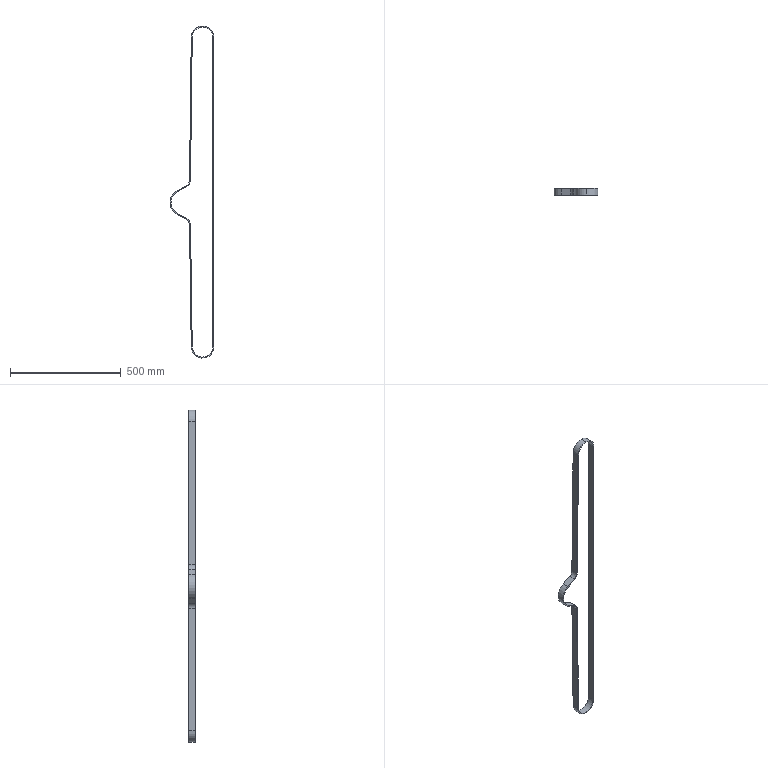Part | SolidWorks | features ExtruThin 1 | 1 solid | 24 faces | box 198.54 x 30 x 1498 mm | volume 429965 mm3 | cylinder 12 | plane 12 | commonest cylinder face diameters 93.49 x3 102.49 x3 55 x2 64 x2 112.59 x1 121.59 x1
STEP:
#1=CARTESIAN_POINT('',(-7.645,219.46,1948.));
#2=VERTEX_POINT('',#1);
#3=CARTESIAN_POINT('',(-54.39,219.46,1994.745));
#4=VERTEX_POINT('',#3);
#5=CARTESIAN_POINT('',(-54.39,219.46,1948.));
#6=DIRECTION('',(0.,-1.,0.));
#7=DIRECTION('',(0.,0.,1.));
#8=AXIS2_PLACEMENT_3D('',#5,#6,#7);
#9=CIRCLE('',#8,46.745);
#10=EDGE_CURVE('',#2,#4,#9,.T.);
#11=ORIENTED_EDGE('',*,*,#10,.T.);
#12=CARTESIAN_POINT('',(-54.39,249.46,1994.745));
#13=VERTEX_POINT('',#12);
#14=CARTESIAN_POINT('',(-54.39,219.46,1994.745));
#15=DIRECTION('',(0.,1.,0.));
#16=VECTOR('',#15,1000.);
#17=LINE('',#14,#16);
#18=EDGE_CURVE('',#4,#13,#17,.T.);
#19=ORIENTED_EDGE('',*,*,#18,.T.);
#20=CARTESIAN_POINT('',(-7.645,249.46,1948.));
#21=VERTEX_POINT('',#20);
#22=CARTESIAN_POINT('',(-54.39,249.46,1948.));
#23=DIRECTION('',(0.,-1.,0.));
#24=DIRECTION('',(0.,0.,1.));
#25=AXIS2_PLACEMENT_3D('',#22,#23,#24);
#26=CIRCLE('',#25,46.745);
#27=EDGE_CURVE('',#21,#13,#26,.T.);
#28=ORIENTED_EDGE('',*,*,#27,.F.);
#29=CARTESIAN_POINT('',(-7.645,219.46,1948.));
#30=DIRECTION('',(0.,1.,0.));
#31=VECTOR('',#30,1000.);
#32=LINE('',#29,#31);
#33=EDGE_CURVE('',#2,#21,#32,.T.);
#34=ORIENTED_EDGE('',*,*,#33,.F.);
#35=EDGE_LOOP('',(#11,#19,#28,#34));
#36=FACE_OUTER_BOUND('',#35,.T.);
#37=CARTESIAN_POINT('',(-54.39,219.46,1948.));
#38=DIRECTION('',(0.,1.,0.));
#39=DIRECTION('',(0.,0.,1.));
#40=AXIS2_PLACEMENT_3D('',#37,#38,#39);
#41=CYLINDRICAL_SURFACE('',#40,46.745);
#42=ADVANCED_FACE('',(#36),#41,.F.);
#43=CARTESIAN_POINT('',(-54.39,219.46,1999.245));
#44=VERTEX_POINT('',#43);
#45=CARTESIAN_POINT('',(-105.631,219.46,1948.615));
#46=VERTEX_POINT('',#45);
#47=CARTESIAN_POINT('',(-54.39,219.46,1948.));
#48=DIRECTION('',(0.,-1.,0.));
#49=DIRECTION('',(0.,0.,1.));
#50=AXIS2_PLACEMENT_3D('',#47,#48,#49);
#51=CIRCLE('',#50,51.245);
#52=EDGE_CURVE('',#44,#46,#51,.T.);
#53=ORIENTED_EDGE('',*,*,#52,.F.);
#54=CARTESIAN_POINT('',(-54.39,249.46,1999.245));
#55=VERTEX_POINT('',#54);
#56=CARTESIAN_POINT('',(-54.39,219.46,1999.245));
#57=DIRECTION('',(0.,1.,0.));
#58=VECTOR('',#57,1000.);
#59=LINE('',#56,#58);
#60=EDGE_CURVE('',#44,#55,#59,.T.);
#61=ORIENTED_EDGE('',*,*,#60,.T.);
#62=CARTESIAN_POINT('',(-105.631,249.46,1948.615));
#63=VERTEX_POINT('',#62);
#64=CARTESIAN_POINT('',(-54.39,249.46,1948.));
#65=DIRECTION('',(0.,-1.,0.));
#66=DIRECTION('',(0.,0.,1.));
#67=AXIS2_PLACEMENT_3D('',#64,#65,#66);
#68=CIRCLE('',#67,51.245);
#69=EDGE_CURVE('',#55,#63,#68,.T.);
#70=ORIENTED_EDGE('',*,*,#69,.T.);
#71=CARTESIAN_POINT('',(-105.631,219.46,1948.615));
#72=DIRECTION('',(0.,1.,0.));
#73=VECTOR('',#72,1000.);
#74=LINE('',#71,#73);
#75=EDGE_CURVE('',#46,#63,#74,.T.);
#76=ORIENTED_EDGE('',*,*,#75,.F.);
#77=EDGE_LOOP('',(#53,#61,#70,#76));
#78=FACE_OUTER_BOUND('',#77,.T.);
#79=CARTESIAN_POINT('',(-54.39,219.46,1948.));
#80=DIRECTION('',(0.,1.,0.));
#81=DIRECTION('',(0.,0.,1.));
#82=AXIS2_PLACEMENT_3D('',#79,#80,#81);
#83=CYLINDRICAL_SURFACE('',#82,51.245);
#84=ADVANCED_FACE('',(#78),#83,.T.);
#85=CARTESIAN_POINT('',(-105.63,219.46,551.279));
#86=VERTEX_POINT('',#85);
#87=CARTESIAN_POINT('',(-3.145,219.46,552.));
#88=VERTEX_POINT('',#87);
#89=CARTESIAN_POINT('',(-54.39,219.46,552.));
#90=DIRECTION('',(0.,-1.,0.));
#91=DIRECTION('',(0.,0.,1.));
#92=AXIS2_PLACEMENT_3D('',#89,#90,#91);
#93=CIRCLE('',#92,51.245);
#94=EDGE_CURVE('',#86,#88,#93,.T.);
#95=ORIENTED_EDGE('',*,*,#94,.T.);
#96=CARTESIAN_POINT('',(-3.145,219.46,1948.));
#97=VERTEX_POINT('',#96);
#98=CARTESIAN_POINT('',(-3.145,219.46,552.));
#99=DIRECTION('',(0.,0.,1.));
#100=VECTOR('',#99,1000.);
#101=LINE('',#98,#100);
#102=EDGE_CURVE('',#88,#97,#101,.T.);
#103=ORIENTED_EDGE('',*,*,#102,.T.);
#104=CARTESIAN_POINT('',(-54.39,219.46,1948.));
#105=DIRECTION('',(0.,-1.,0.));
#106=DIRECTION('',(0.,0.,1.));
#107=AXIS2_PLACEMENT_3D('',#104,#105,#106);
#108=CIRCLE('',#107,51.245);
#109=EDGE_CURVE('',#97,#44,#108,.T.);
#110=ORIENTED_EDGE('',*,*,#109,.T.);
#111=ORIENTED_EDGE('',*,*,#52,.T.);
#112=CARTESIAN_POINT('',(-113.392,219.46,1302.17));
#113=VERTEX_POINT('',#112);
#114=CARTESIAN_POINT('',(-105.631,219.46,1948.615));
#115=DIRECTION('',(-0.012,0.,-0.9999));
#116=VECTOR('',#115,1000.);
#117=LINE('',#114,#116);
#118=EDGE_CURVE('',#46,#113,#117,.T.);
#119=ORIENTED_EDGE('',*,*,#118,.T.);
#120=CARTESIAN_POINT('',(-127.979,219.46,1278.219));
#121=VERTEX_POINT('',#120);
#122=CARTESIAN_POINT('',(-140.89,219.46,1302.5));
#123=DIRECTION('',(0.,1.,0.));
#124=DIRECTION('',(0.,0.,1.));
#125=AXIS2_PLACEMENT_3D('',#122,#123,#124);
#126=CIRCLE('',#125,27.5);
#127=EDGE_CURVE('',#113,#121,#126,.T.);
#128=ORIENTED_EDGE('',*,*,#127,.T.);
#129=CARTESIAN_POINT('',(-169.431,219.46,1256.179));
#130=VERTEX_POINT('',#129);
#131=CARTESIAN_POINT('',(-169.431,219.46,1256.179));
#132=DIRECTION('',(-0.8829,0.,-0.4695));
#133=VECTOR('',#132,1000.);
#134=LINE('',#131,#133);
#135=EDGE_CURVE('',#121,#130,#134,.T.);
#136=ORIENTED_EDGE('',*,*,#135,.T.);
#137=CARTESIAN_POINT('',(-169.431,219.46,1148.821));
#138=VERTEX_POINT('',#137);
#139=CARTESIAN_POINT('',(-140.89,219.46,1202.5));
#140=DIRECTION('',(0.,-1.,0.));
#141=DIRECTION('',(0.,0.,1.));
#142=AXIS2_PLACEMENT_3D('',#139,#140,#141);
#143=CIRCLE('',#142,60.795);
#144=EDGE_CURVE('',#130,#138,#143,.T.);
#145=ORIENTED_EDGE('',*,*,#144,.T.);
#146=CARTESIAN_POINT('',(-127.979,219.46,1126.781));
#147=VERTEX_POINT('',#146);
#148=CARTESIAN_POINT('',(-127.979,219.46,1126.781));
#149=DIRECTION('',(0.883,0.,-0.4695));
#150=VECTOR('',#149,1000.);
#151=LINE('',#148,#150);
#152=EDGE_CURVE('',#138,#147,#151,.T.);
#153=ORIENTED_EDGE('',*,*,#152,.T.);
#154=CARTESIAN_POINT('',(-113.393,219.46,1102.887));
#155=VERTEX_POINT('',#154);
#156=CARTESIAN_POINT('',(-140.89,219.46,1102.5));
#157=DIRECTION('',(0.,1.,0.));
#158=DIRECTION('',(0.,0.,1.));
#159=AXIS2_PLACEMENT_3D('',#156,#157,#158);
#160=CIRCLE('',#159,27.5);
#161=EDGE_CURVE('',#147,#155,#160,.T.);
#162=ORIENTED_EDGE('',*,*,#161,.T.);
#163=CARTESIAN_POINT('',(-105.63,219.46,551.279));
#164=DIRECTION('',(0.01407,0.,-0.9999));
#165=VECTOR('',#164,1000.);
#166=LINE('',#163,#165);
#167=EDGE_CURVE('',#155,#86,#166,.T.);
#168=ORIENTED_EDGE('',*,*,#167,.T.);
#169=EDGE_LOOP('',(#95,#103,#110,#111,#119,#128,#136,#145,#153,#162,#168));
#170=FACE_OUTER_BOUND('',#169,.T.);
#171=CARTESIAN_POINT('',(-7.645,219.46,552.));
#172=VERTEX_POINT('',#171);
#173=CARTESIAN_POINT('',(-7.645,219.46,552.));
#174=DIRECTION('',(0.,0.,1.));
#175=VECTOR('',#174,1000.);
#176=LINE('',#173,#175);
#177=EDGE_CURVE('',#172,#2,#176,.T.);
#178=ORIENTED_EDGE('',*,*,#177,.F.);
#179=CARTESIAN_POINT('',(-101.13,219.46,551.342));
#180=VERTEX_POINT('',#179);
#181=CARTESIAN_POINT('',(-54.39,219.46,552.));
#182=DIRECTION('',(0.,-1.,0.));
#183=DIRECTION('',(0.,0.,1.));
#184=AXIS2_PLACEMENT_3D('',#181,#182,#183);
#185=CIRCLE('',#184,46.745);
#186=EDGE_CURVE('',#180,#172,#185,.T.);
#187=ORIENTED_EDGE('',*,*,#186,.F.);
#188=CARTESIAN_POINT('',(-108.893,219.46,1102.95));
#189=VERTEX_POINT('',#188);
#190=CARTESIAN_POINT('',(-101.13,219.46,551.342));
#191=DIRECTION('',(0.01407,0.,-0.9999));
#192=VECTOR('',#191,1000.);
#193=LINE('',#190,#192);
#194=EDGE_CURVE('',#189,#180,#193,.T.);
#195=ORIENTED_EDGE('',*,*,#194,.F.);
#196=CARTESIAN_POINT('',(-125.867,219.46,1130.754));
#197=VERTEX_POINT('',#196);
#198=CARTESIAN_POINT('',(-140.89,219.46,1102.5));
#199=DIRECTION('',(0.,1.,0.));
#200=DIRECTION('',(0.,0.,1.));
#201=AXIS2_PLACEMENT_3D('',#198,#199,#200);
#202=CIRCLE('',#201,32.);
#203=EDGE_CURVE('',#197,#189,#202,.T.);
#204=ORIENTED_EDGE('',*,*,#203,.F.);
#205=CARTESIAN_POINT('',(-167.318,219.46,1152.794));
#206=VERTEX_POINT('',#205);
#207=CARTESIAN_POINT('',(-125.867,219.46,1130.754));
#208=DIRECTION('',(0.883,0.,-0.4695));
#209=VECTOR('',#208,1000.);
#210=LINE('',#207,#209);
#211=EDGE_CURVE('',#206,#197,#210,.T.);
#212=ORIENTED_EDGE('',*,*,#211,.F.);
#213=CARTESIAN_POINT('',(-167.318,219.46,1252.206));
#214=VERTEX_POINT('',#213);
#215=CARTESIAN_POINT('',(-140.89,219.46,1202.5));
#216=DIRECTION('',(0.,-1.,0.));
#217=DIRECTION('',(0.,0.,1.));
#218=AXIS2_PLACEMENT_3D('',#215,#216,#217);
#219=CIRCLE('',#218,56.295);
#220=EDGE_CURVE('',#214,#206,#219,.T.);
#221=ORIENTED_EDGE('',*,*,#220,.F.);
#222=CARTESIAN_POINT('',(-125.867,219.46,1274.246));
#223=VERTEX_POINT('',#222);
#224=CARTESIAN_POINT('',(-167.318,219.46,1252.206));
#225=DIRECTION('',(-0.8829,0.,-0.4695));
#226=VECTOR('',#225,1000.);
#227=LINE('',#224,#226);
#228=EDGE_CURVE('',#223,#214,#227,.T.);
#229=ORIENTED_EDGE('',*,*,#228,.F.);
#230=CARTESIAN_POINT('',(-108.892,219.46,1302.116));
#231=VERTEX_POINT('',#230);
#232=CARTESIAN_POINT('',(-140.89,219.46,1302.5));
#233=DIRECTION('',(0.,1.,0.));
#234=DIRECTION('',(0.,0.,1.));
#235=AXIS2_PLACEMENT_3D('',#232,#233,#234);
#236=CIRCLE('',#235,32.);
#237=EDGE_CURVE('',#231,#223,#236,.T.);
#238=ORIENTED_EDGE('',*,*,#237,.F.);
#239=CARTESIAN_POINT('',(-101.131,219.46,1948.561));
#240=VERTEX_POINT('',#239);
#241=CARTESIAN_POINT('',(-101.131,219.46,1948.561));
#242=DIRECTION('',(-0.012,0.,-0.9999));
#243=VECTOR('',#242,1000.);
#244=LINE('',#241,#243);
#245=EDGE_CURVE('',#240,#231,#244,.T.);
#246=ORIENTED_EDGE('',*,*,#245,.F.);
#247=CARTESIAN_POINT('',(-54.39,219.46,1948.));
#248=DIRECTION('',(0.,-1.,0.));
#249=DIRECTION('',(0.,0.,1.));
#250=AXIS2_PLACEMENT_3D('',#247,#248,#249);
#251=CIRCLE('',#250,46.745);
#252=EDGE_CURVE('',#4,#240,#251,.T.);
#253=ORIENTED_EDGE('',*,*,#252,.F.);
#254=ORIENTED_EDGE('',*,*,#10,.F.);
#255=EDGE_LOOP('',(#178,#187,#195,#204,#212,#221,#229,#238,#246,#253,#254));
#256=FACE_BOUND('',#255,.T.);
#257=CARTESIAN_POINT('',(-54.39,219.46,552.));
#258=DIRECTION('',(0.,-1.,0.));
#259=DIRECTION('',(0.,0.,-1.));
#260=AXIS2_PLACEMENT_3D('',#257,#258,#259);
#261=PLANE('',#260);
#262=ADVANCED_FACE('',(#170,#256),#261,.T.);
#263=CARTESIAN_POINT('',(-105.63,249.46,551.279));
#264=VERTEX_POINT('',#263);
#265=CARTESIAN_POINT('',(-3.145,249.46,552.));
#266=VERTEX_POINT('',#265);
#267=CARTESIAN_POINT('',(-54.39,249.46,552.));
#268=DIRECTION('',(0.,-1.,0.));
#269=DIRECTION('',(0.,0.,1.));
#270=AXIS2_PLACEMENT_3D('',#267,#268,#269);
#271=CIRCLE('',#270,51.245);
#272=EDGE_CURVE('',#264,#266,#271,.T.);
#273=ORIENTED_EDGE('',*,*,#272,.F.);
#274=CARTESIAN_POINT('',(-113.393,249.46,1102.887));
#275=VERTEX_POINT('',#274);
#276=CARTESIAN_POINT('',(-105.63,249.46,551.279));
#277=DIRECTION('',(0.01407,0.,-0.9999));
#278=VECTOR('',#277,1000.);
#279=LINE('',#276,#278);
#280=EDGE_CURVE('',#275,#264,#279,.T.);
#281=ORIENTED_EDGE('',*,*,#280,.F.);
#282=CARTESIAN_POINT('',(-127.979,249.46,1126.781));
#283=VERTEX_POINT('',#282);
#284=CARTESIAN_POINT('',(-140.89,249.46,1102.5));
#285=DIRECTION('',(0.,1.,0.));
#286=DIRECTION('',(0.,0.,1.));
#287=AXIS2_PLACEMENT_3D('',#284,#285,#286);
#288=CIRCLE('',#287,27.5);
#289=EDGE_CURVE('',#283,#275,#288,.T.);
#290=ORIENTED_EDGE('',*,*,#289,.F.);
#291=CARTESIAN_POINT('',(-169.431,249.46,1148.821));
#292=VERTEX_POINT('',#291);
#293=CARTESIAN_POINT('',(-127.979,249.46,1126.781));
#294=DIRECTION('',(0.883,0.,-0.4695));
#295=VECTOR('',#294,1000.);
#296=LINE('',#293,#295);
#297=EDGE_CURVE('',#292,#283,#296,.T.);
#298=ORIENTED_EDGE('',*,*,#297,.F.);
#299=CARTESIAN_POINT('',(-169.431,249.46,1256.179));
#300=VERTEX_POINT('',#299);
#301=CARTESIAN_POINT('',(-140.89,249.46,1202.5));
#302=DIRECTION('',(0.,-1.,0.));
#303=DIRECTION('',(0.,0.,1.));
#304=AXIS2_PLACEMENT_3D('',#301,#302,#303);
#305=CIRCLE('',#304,60.795);
#306=EDGE_CURVE('',#300,#292,#305,.T.);
#307=ORIENTED_EDGE('',*,*,#306,.F.);
#308=CARTESIAN_POINT('',(-127.979,249.46,1278.219));
#309=VERTEX_POINT('',#308);
#310=CARTESIAN_POINT('',(-169.431,249.46,1256.179));
#311=DIRECTION('',(-0.8829,0.,-0.4695));
#312=VECTOR('',#311,1000.);
#313=LINE('',#310,#312);
#314=EDGE_CURVE('',#309,#300,#313,.T.);
#315=ORIENTED_EDGE('',*,*,#314,.F.);
#316=CARTESIAN_POINT('',(-113.392,249.46,1302.17));
#317=VERTEX_POINT('',#316);
#318=CARTESIAN_POINT('',(-140.89,249.46,1302.5));
#319=DIRECTION('',(0.,1.,0.));
#320=DIRECTION('',(0.,0.,1.));
#321=AXIS2_PLACEMENT_3D('',#318,#319,#320);
#322=CIRCLE('',#321,27.5);
#323=EDGE_CURVE('',#317,#309,#322,.T.);
#324=ORIENTED_EDGE('',*,*,#323,.F.);
#325=CARTESIAN_POINT('',(-105.631,249.46,1948.615));
#326=DIRECTION('',(-0.012,0.,-0.9999));
#327=VECTOR('',#326,1000.);
#328=LINE('',#325,#327);
#329=EDGE_CURVE('',#63,#317,#328,.T.);
#330=ORIENTED_EDGE('',*,*,#329,.F.);
#331=ORIENTED_EDGE('',*,*,#69,.F.);
#332=CARTESIAN_POINT('',(-3.145,249.46,1948.));
#333=VERTEX_POINT('',#332);
#334=CARTESIAN_POINT('',(-54.39,249.46,1948.));
#335=DIRECTION('',(0.,-1.,0.));
#336=DIRECTION('',(0.,0.,1.));
#337=AXIS2_PLACEMENT_3D('',#334,#335,#336);
#338=CIRCLE('',#337,51.245);
#339=EDGE_CURVE('',#333,#55,#338,.T.);
#340=ORIENTED_EDGE('',*,*,#339,.F.);
#341=CARTESIAN_POINT('',(-3.145,249.46,552.));
#342=DIRECTION('',(0.,0.,1.));
#343=VECTOR('',#342,1000.);
#344=LINE('',#341,#343);
#345=EDGE_CURVE('',#266,#333,#344,.T.);
#346=ORIENTED_EDGE('',*,*,#345,.F.);
#347=EDGE_LOOP('',(#273,#281,#290,#298,#307,#315,#324,#330,#331,#340,#346));
#348=FACE_OUTER_BOUND('',#347,.T.);
#349=CARTESIAN_POINT('',(-101.13,249.46,551.342));
#350=VERTEX_POINT('',#349);
#351=CARTESIAN_POINT('',(-7.645,249.46,552.));
#352=VERTEX_POINT('',#351);
#353=CARTESIAN_POINT('',(-54.39,249.46,552.));
#354=DIRECTION('',(0.,-1.,0.));
#355=DIRECTION('',(0.,0.,1.));
#356=AXIS2_PLACEMENT_3D('',#353,#354,#355);
#357=CIRCLE('',#356,46.745);
#358=EDGE_CURVE('',#350,#352,#357,.T.);
#359=ORIENTED_EDGE('',*,*,#358,.T.);
#360=CARTESIAN_POINT('',(-7.645,249.46,552.));
#361=DIRECTION('',(0.,0.,1.));
#362=VECTOR('',#361,1000.);
#363=LINE('',#360,#362);
#364=EDGE_CURVE('',#352,#21,#363,.T.);
#365=ORIENTED_EDGE('',*,*,#364,.T.);
#366=ORIENTED_EDGE('',*,*,#27,.T.);
#367=CARTESIAN_POINT('',(-101.131,249.46,1948.561));
#368=VERTEX_POINT('',#367);
#369=CARTESIAN_POINT('',(-54.39,249.46,1948.));
#370=DIRECTION('',(0.,-1.,0.));
#371=DIRECTION('',(0.,0.,1.));
#372=AXIS2_PLACEMENT_3D('',#369,#370,#371);
#373=CIRCLE('',#372,46.745);
#374=EDGE_CURVE('',#13,#368,#373,.T.);
#375=ORIENTED_EDGE('',*,*,#374,.T.);
#376=CARTESIAN_POINT('',(-108.892,249.46,1302.116));
#377=VERTEX_POINT('',#376);
#378=CARTESIAN_POINT('',(-101.131,249.46,1948.561));
#379=DIRECTION('',(-0.012,0.,-0.9999));
#380=VECTOR('',#379,1000.);
#381=LINE('',#378,#380);
#382=EDGE_CURVE('',#368,#377,#381,.T.);
#383=ORIENTED_EDGE('',*,*,#382,.T.);
#384=CARTESIAN_POINT('',(-125.867,249.46,1274.246));
#385=VERTEX_POINT('',#384);
#386=CARTESIAN_POINT('',(-140.89,249.46,1302.5));
#387=DIRECTION('',(0.,1.,0.));
#388=DIRECTION('',(0.,0.,1.));
#389=AXIS2_PLACEMENT_3D('',#386,#387,#388);
#390=CIRCLE('',#389,32.);
#391=EDGE_CURVE('',#377,#385,#390,.T.);
#392=ORIENTED_EDGE('',*,*,#391,.T.);
#393=CARTESIAN_POINT('',(-167.318,249.46,1252.206));
#394=VERTEX_POINT('',#393);
#395=CARTESIAN_POINT('',(-167.318,249.46,1252.206));
#396=DIRECTION('',(-0.8829,0.,-0.4695));
#397=VECTOR('',#396,1000.);
#398=LINE('',#395,#397);
#399=EDGE_CURVE('',#385,#394,#398,.T.);
#400=ORIENTED_EDGE('',*,*,#399,.T.);
#401=CARTESIAN_POINT('',(-167.318,249.46,1152.794));
#402=VERTEX_POINT('',#401);
#403=CARTESIAN_POINT('',(-140.89,249.46,1202.5));
#404=DIRECTION('',(0.,-1.,0.));
#405=DIRECTION('',(0.,0.,1.));
#406=AXIS2_PLACEMENT_3D('',#403,#404,#405);
#407=CIRCLE('',#406,56.295);
#408=EDGE_CURVE('',#394,#402,#407,.T.);
#409=ORIENTED_EDGE('',*,*,#408,.T.);
#410=CARTESIAN_POINT('',(-125.867,249.46,1130.754));
#411=VERTEX_POINT('',#410);
#412=CARTESIAN_POINT('',(-125.867,249.46,1130.754));
#413=DIRECTION('',(0.883,0.,-0.4695));
#414=VECTOR('',#413,1000.);
#415=LINE('',#412,#414);
#416=EDGE_CURVE('',#402,#411,#415,.T.);
#417=ORIENTED_EDGE('',*,*,#416,.T.);
#418=CARTESIAN_POINT('',(-108.893,249.46,1102.95));
#419=VERTEX_POINT('',#418);
#420=CARTESIAN_POINT('',(-140.89,249.46,1102.5));
#421=DIRECTION('',(0.,1.,0.));
#422=DIRECTION('',(0.,0.,1.));
#423=AXIS2_PLACEMENT_3D('',#420,#421,#422);
#424=CIRCLE('',#423,32.);
#425=EDGE_CURVE('',#411,#419,#424,.T.);
#426=ORIENTED_EDGE('',*,*,#425,.T.);
#427=CARTESIAN_POINT('',(-101.13,249.46,551.342));
#428=DIRECTION('',(0.01407,0.,-0.9999));
#429=VECTOR('',#428,1000.);
#430=LINE('',#427,#429);
#431=EDGE_CURVE('',#419,#350,#430,.T.);
#432=ORIENTED_EDGE('',*,*,#431,.T.);
#433=EDGE_LOOP('',(#359,#365,#366,#375,#383,#392,#400,#409,#417,#426,#432));
#434=FACE_BOUND('',#433,.T.);
#435=CARTESIAN_POINT('',(-54.39,249.46,552.));
#436=DIRECTION('',(0.,-1.,0.));
#437=DIRECTION('',(0.,0.,-1.));
#438=AXIS2_PLACEMENT_3D('',#435,#436,#437);
#439=PLANE('',#438);
#440=ADVANCED_FACE('',(#348,#434),#439,.F.);
#441=ORIENTED_EDGE('',*,*,#272,.T.);
#442=CARTESIAN_POINT('',(-3.145,219.46,552.));
#443=DIRECTION('',(0.,1.,0.));
#444=VECTOR('',#443,1000.);
#445=LINE('',#442,#444);
#446=EDGE_CURVE('',#88,#266,#445,.T.);
#447=ORIENTED_EDGE('',*,*,#446,.F.);
#448=ORIENTED_EDGE('',*,*,#94,.F.);
#449=CARTESIAN_POINT('',(-105.63,219.46,551.279));
#450=DIRECTION('',(0.,1.,0.));
#451=VECTOR('',#450,1000.);
#452=LINE('',#449,#451);
#453=EDGE_CURVE('',#86,#264,#452,.T.);
#454=ORIENTED_EDGE('',*,*,#453,.T.);
#455=EDGE_LOOP('',(#441,#447,#448,#454));
#456=FACE_OUTER_BOUND('',#455,.T.);
#457=CARTESIAN_POINT('',(-54.39,219.46,552.));
#458=DIRECTION('',(0.,1.,0.));
#459=DIRECTION('',(0.,0.,1.));
#460=AXIS2_PLACEMENT_3D('',#457,#458,#459);
#461=CYLINDRICAL_SURFACE('',#460,51.245);
#462=ADVANCED_FACE('',(#456),#461,.T.);
#463=ORIENTED_EDGE('',*,*,#345,.T.);
#464=CARTESIAN_POINT('',(-3.145,219.46,1948.));
#465=DIRECTION('',(0.,1.,0.));
#466=VECTOR('',#465,1000.);
#467=LINE('',#464,#466);
#468=EDGE_CURVE('',#97,#333,#467,.T.);
#469=ORIENTED_EDGE('',*,*,#468,.F.);
#470=ORIENTED_EDGE('',*,*,#102,.F.);
#471=ORIENTED_EDGE('',*,*,#446,.T.);
#472=EDGE_LOOP('',(#463,#469,#470,#471));
#473=FACE_OUTER_BOUND('',#472,.T.);
#474=CARTESIAN_POINT('',(-3.145,219.46,552.));
#475=DIRECTION('',(-1.,0.,0.));
#476=DIRECTION('',(0.,-1.,0.));
#477=AXIS2_PLACEMENT_3D('',#474,#475,#476);
#478=PLANE('',#477);
#479=ADVANCED_FACE('',(#473),#478,.F.);
#480=ORIENTED_EDGE('',*,*,#60,.F.);
#481=ORIENTED_EDGE('',*,*,#109,.F.);
#482=ORIENTED_EDGE('',*,*,#468,.T.);
#483=ORIENTED_EDGE('',*,*,#339,.T.);
#484=EDGE_LOOP('',(#480,#481,#482,#483));
#485=FACE_OUTER_BOUND('',#484,.T.);
#486=CARTESIAN_POINT('',(-54.39,219.46,1948.));
#487=DIRECTION('',(0.,1.,0.));
#488=DIRECTION('',(0.,0.,1.));
#489=AXIS2_PLACEMENT_3D('',#486,#487,#488);
#490=CYLINDRICAL_SURFACE('',#489,51.245);
#491=ADVANCED_FACE('',(#485),#490,.T.);
#492=ORIENTED_EDGE('',*,*,#329,.T.);
#493=CARTESIAN_POINT('',(-113.392,219.46,1302.17));
#494=DIRECTION('',(0.,1.,0.));
#495=VECTOR('',#494,1000.);
#496=LINE('',#493,#495);
#497=EDGE_CURVE('',#113,#317,#496,.T.);
#498=ORIENTED_EDGE('',*,*,#497,.F.);
#499=ORIENTED_EDGE('',*,*,#118,.F.);
#500=ORIENTED_EDGE('',*,*,#75,.T.);
#501=EDGE_LOOP('',(#492,#498,#499,#500));
#502=FACE_OUTER_BOUND('',#501,.T.);
#503=CARTESIAN_POINT('',(-105.631,219.46,1948.615));
#504=DIRECTION('',(0.9999,0.,-0.012));
#505=DIRECTION('',(-0.012,0.,-0.9999));
#506=AXIS2_PLACEMENT_3D('',#503,#504,#505);
#507=PLANE('',#506);
#508=ADVANCED_FACE('',(#502),#507,.F.);
#509=ORIENTED_EDGE('',*,*,#323,.T.);
#510=CARTESIAN_POINT('',(-127.979,219.46,1278.219));
#511=DIRECTION('',(0.,1.,0.));
#512=VECTOR('',#511,1000.);
#513=LINE('',#510,#512);
#514=EDGE_CURVE('',#121,#309,#513,.T.);
#515=ORIENTED_EDGE('',*,*,#514,.F.);
#516=ORIENTED_EDGE('',*,*,#127,.F.);
#517=ORIENTED_EDGE('',*,*,#497,.T.);
#518=EDGE_LOOP('',(#509,#515,#516,#517));
#519=FACE_OUTER_BOUND('',#518,.T.);
#520=CARTESIAN_POINT('',(-140.89,219.46,1302.5));
#521=DIRECTION('',(0.,1.,0.));
#522=DIRECTION('',(0.,0.,1.));
#523=AXIS2_PLACEMENT_3D('',#520,#521,#522);
#524=CYLINDRICAL_SURFACE('',#523,27.5);
#525=ADVANCED_FACE('',(#519),#524,.F.);
#526=ORIENTED_EDGE('',*,*,#314,.T.);
#527=CARTESIAN_POINT('',(-169.431,219.46,1256.179));
#528=DIRECTION('',(0.,1.,0.));
#529=VECTOR('',#528,1000.);
#530=LINE('',#527,#529);
#531=EDGE_CURVE('',#130,#300,#530,.T.);
#532=ORIENTED_EDGE('',*,*,#531,.F.);
#533=ORIENTED_EDGE('',*,*,#135,.F.);
#534=ORIENTED_EDGE('',*,*,#514,.T.);
#535=EDGE_LOOP('',(#526,#532,#533,#534));
#536=FACE_OUTER_BOUND('',#535,.T.);
#537=CARTESIAN_POINT('',(-169.431,219.46,1256.179));
#538=DIRECTION('',(0.4695,0.,-0.8829));
#539=DIRECTION('',(-0.8829,0.,-0.4695));
#540=AXIS2_PLACEMENT_3D('',#537,#538,#539);
#541=PLANE('',#540);
#542=ADVANCED_FACE('',(#536),#541,.F.);
#543=ORIENTED_EDGE('',*,*,#306,.T.);
#544=CARTESIAN_POINT('',(-169.431,219.46,1148.821));
#545=DIRECTION('',(0.,1.,0.));
#546=VECTOR('',#545,1000.);
#547=LINE('',#544,#546);
#548=EDGE_CURVE('',#138,#292,#547,.T.);
#549=ORIENTED_EDGE('',*,*,#548,.F.);
#550=ORIENTED_EDGE('',*,*,#144,.F.);
#551=ORIENTED_EDGE('',*,*,#531,.T.);
#552=EDGE_LOOP('',(#543,#549,#550,#551));
#553=FACE_OUTER_BOUND('',#552,.T.);
#554=CARTESIAN_POINT('',(-140.89,219.46,1202.5));
#555=DIRECTION('',(0.,1.,0.));
#556=DIRECTION('',(0.,0.,1.));
#557=AXIS2_PLACEMENT_3D('',#554,#555,#556);
#558=CYLINDRICAL_SURFACE('',#557,60.795);
#559=ADVANCED_FACE('',(#553),#558,.T.);
#560=ORIENTED_EDGE('',*,*,#297,.T.);
#561=CARTESIAN_POINT('',(-127.979,219.46,1126.781));
#562=DIRECTION('',(0.,1.,0.));
#563=VECTOR('',#562,1000.);
#564=LINE('',#561,#563);
#565=EDGE_CURVE('',#147,#283,#564,.T.);
#566=ORIENTED_EDGE('',*,*,#565,.F.);
#567=ORIENTED_EDGE('',*,*,#152,.F.);
#568=ORIENTED_EDGE('',*,*,#548,.T.);
#569=EDGE_LOOP('',(#560,#566,#567,#568));
#570=FACE_OUTER_BOUND('',#569,.T.);
#571=CARTESIAN_POINT('',(-127.979,219.46,1126.781));
#572=DIRECTION('',(0.4695,0.,0.883));
#573=DIRECTION('',(0.883,0.,-0.4695));
#574=AXIS2_PLACEMENT_3D('',#571,#572,#573);
#575=PLANE('',#574);
#576=ADVANCED_FACE('',(#570),#575,.F.);
#577=ORIENTED_EDGE('',*,*,#289,.T.);
#578=CARTESIAN_POINT('',(-113.393,219.46,1102.887));
#579=DIRECTION('',(0.,1.,0.));
#580=VECTOR('',#579,1000.);
#581=LINE('',#578,#580);
#582=EDGE_CURVE('',#155,#275,#581,.T.);
#583=ORIENTED_EDGE('',*,*,#582,.F.);
#584=ORIENTED_EDGE('',*,*,#161,.F.);
#585=ORIENTED_EDGE('',*,*,#565,.T.);
#586=EDGE_LOOP('',(#577,#583,#584,#585));
#587=FACE_OUTER_BOUND('',#586,.T.);
#588=CARTESIAN_POINT('',(-140.89,219.46,1102.5));
#589=DIRECTION('',(0.,1.,0.));
#590=DIRECTION('',(0.,0.,1.));
#591=AXIS2_PLACEMENT_3D('',#588,#589,#590);
#592=CYLINDRICAL_SURFACE('',#591,27.5);
#593=ADVANCED_FACE('',(#587),#592,.F.);
#594=ORIENTED_EDGE('',*,*,#280,.T.);
#595=ORIENTED_EDGE('',*,*,#453,.F.);
#596=ORIENTED_EDGE('',*,*,#167,.F.);
#597=ORIENTED_EDGE('',*,*,#582,.T.);
#598=EDGE_LOOP('',(#594,#595,#596,#597));
#599=FACE_OUTER_BOUND('',#598,.T.);
#600=CARTESIAN_POINT('',(-105.63,219.46,551.279));
#601=DIRECTION('',(0.9999,0.,0.01407));
#602=DIRECTION('',(0.01407,0.,-0.9999));
#603=AXIS2_PLACEMENT_3D('',#600,#601,#602);
#604=PLANE('',#603);
#605=ADVANCED_FACE('',(#599),#604,.F.);
#606=ORIENTED_EDGE('',*,*,#358,.F.);
#607=CARTESIAN_POINT('',(-101.13,219.46,551.342));
#608=DIRECTION('',(0.,1.,0.));
#609=VECTOR('',#608,1000.);
#610=LINE('',#607,#609);
#611=EDGE_CURVE('',#180,#350,#610,.T.);
#612=ORIENTED_EDGE('',*,*,#611,.F.);
#613=ORIENTED_EDGE('',*,*,#186,.T.);
#614=CARTESIAN_POINT('',(-7.645,219.46,552.));
#615=DIRECTION('',(0.,1.,0.));
#616=VECTOR('',#615,1000.);
#617=LINE('',#614,#616);
#618=EDGE_CURVE('',#172,#352,#617,.T.);
#619=ORIENTED_EDGE('',*,*,#618,.T.);
#620=EDGE_LOOP('',(#606,#612,#613,#619));
#621=FACE_OUTER_BOUND('',#620,.T.);
#622=CARTESIAN_POINT('',(-54.39,219.46,552.));
#623=DIRECTION('',(0.,1.,0.));
#624=DIRECTION('',(0.,0.,1.));
#625=AXIS2_PLACEMENT_3D('',#622,#623,#624);
#626=CYLINDRICAL_SURFACE('',#625,46.745);
#627=ADVANCED_FACE('',(#621),#626,.F.);
#628=ORIENTED_EDGE('',*,*,#364,.F.);
#629=ORIENTED_EDGE('',*,*,#618,.F.);
#630=ORIENTED_EDGE('',*,*,#177,.T.);
#631=ORIENTED_EDGE('',*,*,#33,.T.);
#632=EDGE_LOOP('',(#628,#629,#630,#631));
#633=FACE_OUTER_BOUND('',#632,.T.);
#634=CARTESIAN_POINT('',(-7.645,219.46,552.));
#635=DIRECTION('',(-1.,0.,0.));
#636=DIRECTION('',(0.,-1.,0.));
#637=AXIS2_PLACEMENT_3D('',#634,#635,#636);
#638=PLANE('',#637);
#639=ADVANCED_FACE('',(#633),#638,.T.);
#640=ORIENTED_EDGE('',*,*,#18,.F.);
#641=ORIENTED_EDGE('',*,*,#252,.T.);
#642=CARTESIAN_POINT('',(-101.131,219.46,1948.561));
#643=DIRECTION('',(0.,1.,0.));
#644=VECTOR('',#643,1000.);
#645=LINE('',#642,#644);
#646=EDGE_CURVE('',#240,#368,#645,.T.);
#647=ORIENTED_EDGE('',*,*,#646,.T.);
#648=ORIENTED_EDGE('',*,*,#374,.F.);
#649=EDGE_LOOP('',(#640,#641,#647,#648));
#650=FACE_OUTER_BOUND('',#649,.T.);
#651=CARTESIAN_POINT('',(-54.39,219.46,1948.));
#652=DIRECTION('',(0.,1.,0.));
#653=DIRECTION('',(0.,0.,1.));
#654=AXIS2_PLACEMENT_3D('',#651,#652,#653);
#655=CYLINDRICAL_SURFACE('',#654,46.745);
#656=ADVANCED_FACE('',(#650),#655,.F.);
#657=ORIENTED_EDGE('',*,*,#382,.F.);
#658=ORIENTED_EDGE('',*,*,#646,.F.);
#659=ORIENTED_EDGE('',*,*,#245,.T.);
#660=CARTESIAN_POINT('',(-108.892,219.46,1302.116));
#661=DIRECTION('',(0.,1.,0.));
#662=VECTOR('',#661,1000.);
#663=LINE('',#660,#662);
#664=EDGE_CURVE('',#231,#377,#663,.T.);
#665=ORIENTED_EDGE('',*,*,#664,.T.);
#666=EDGE_LOOP('',(#657,#658,#659,#665));
#667=FACE_OUTER_BOUND('',#666,.T.);
#668=CARTESIAN_POINT('',(-101.131,219.46,1948.561));
#669=DIRECTION('',(0.9999,0.,-0.012));
#670=DIRECTION('',(-0.012,0.,-0.9999));
#671=AXIS2_PLACEMENT_3D('',#668,#669,#670);
#672=PLANE('',#671);
#673=ADVANCED_FACE('',(#667),#672,.T.);
#674=ORIENTED_EDGE('',*,*,#391,.F.);
#675=ORIENTED_EDGE('',*,*,#664,.F.);
#676=ORIENTED_EDGE('',*,*,#237,.T.);
#677=CARTESIAN_POINT('',(-125.867,219.46,1274.246));
#678=DIRECTION('',(0.,1.,0.));
#679=VECTOR('',#678,1000.);
#680=LINE('',#677,#679);
#681=EDGE_CURVE('',#223,#385,#680,.T.);
#682=ORIENTED_EDGE('',*,*,#681,.T.);
#683=EDGE_LOOP('',(#674,#675,#676,#682));
#684=FACE_OUTER_BOUND('',#683,.T.);
#685=CARTESIAN_POINT('',(-140.89,219.46,1302.5));
#686=DIRECTION('',(0.,1.,0.));
#687=DIRECTION('',(0.,0.,1.));
#688=AXIS2_PLACEMENT_3D('',#685,#686,#687);
#689=CYLINDRICAL_SURFACE('',#688,32.);
#690=ADVANCED_FACE('',(#684),#689,.T.);
#691=ORIENTED_EDGE('',*,*,#399,.F.);
#692=ORIENTED_EDGE('',*,*,#681,.F.);
#693=ORIENTED_EDGE('',*,*,#228,.T.);
#694=CARTESIAN_POINT('',(-167.318,219.46,1252.206));
#695=DIRECTION('',(0.,1.,0.));
#696=VECTOR('',#695,1000.);
#697=LINE('',#694,#696);
#698=EDGE_CURVE('',#214,#394,#697,.T.);
#699=ORIENTED_EDGE('',*,*,#698,.T.);
#700=EDGE_LOOP('',(#691,#692,#693,#699));
#701=FACE_OUTER_BOUND('',#700,.T.);
#702=CARTESIAN_POINT('',(-167.318,219.46,1252.206));
#703=DIRECTION('',(0.4695,0.,-0.8829));
#704=DIRECTION('',(-0.8829,0.,-0.4695));
#705=AXIS2_PLACEMENT_3D('',#702,#703,#704);
#706=PLANE('',#705);
#707=ADVANCED_FACE('',(#701),#706,.T.);
#708=ORIENTED_EDGE('',*,*,#408,.F.);
#709=ORIENTED_EDGE('',*,*,#698,.F.);
#710=ORIENTED_EDGE('',*,*,#220,.T.);
#711=CARTESIAN_POINT('',(-167.318,219.46,1152.794));
#712=DIRECTION('',(0.,1.,0.));
#713=VECTOR('',#712,1000.);
#714=LINE('',#711,#713);
#715=EDGE_CURVE('',#206,#402,#714,.T.);
#716=ORIENTED_EDGE('',*,*,#715,.T.);
#717=EDGE_LOOP('',(#708,#709,#710,#716));
#718=FACE_OUTER_BOUND('',#717,.T.);
#719=CARTESIAN_POINT('',(-140.89,219.46,1202.5));
#720=DIRECTION('',(0.,1.,0.));
#721=DIRECTION('',(0.,0.,1.));
#722=AXIS2_PLACEMENT_3D('',#719,#720,#721);
#723=CYLINDRICAL_SURFACE('',#722,56.295);
#724=ADVANCED_FACE('',(#718),#723,.F.);
#725=ORIENTED_EDGE('',*,*,#416,.F.);
#726=ORIENTED_EDGE('',*,*,#715,.F.);
#727=ORIENTED_EDGE('',*,*,#211,.T.);
#728=CARTESIAN_POINT('',(-125.867,219.46,1130.754));
#729=DIRECTION('',(0.,1.,0.));
#730=VECTOR('',#729,1000.);
#731=LINE('',#728,#730);
#732=EDGE_CURVE('',#197,#411,#731,.T.);
#733=ORIENTED_EDGE('',*,*,#732,.T.);
#734=EDGE_LOOP('',(#725,#726,#727,#733));
#735=FACE_OUTER_BOUND('',#734,.T.);
#736=CARTESIAN_POINT('',(-125.867,219.46,1130.754));
#737=DIRECTION('',(0.4695,0.,0.883));
#738=DIRECTION('',(0.883,0.,-0.4695));
#739=AXIS2_PLACEMENT_3D('',#736,#737,#738);
#740=PLANE('',#739);
#741=ADVANCED_FACE('',(#735),#740,.T.);
#742=ORIENTED_EDGE('',*,*,#425,.F.);
#743=ORIENTED_EDGE('',*,*,#732,.F.);
#744=ORIENTED_EDGE('',*,*,#203,.T.);
#745=CARTESIAN_POINT('',(-108.893,219.46,1102.95));
#746=DIRECTION('',(0.,1.,0.));
#747=VECTOR('',#746,1000.);
#748=LINE('',#745,#747);
#749=EDGE_CURVE('',#189,#419,#748,.T.);
#750=ORIENTED_EDGE('',*,*,#749,.T.);
#751=EDGE_LOOP('',(#742,#743,#744,#750));
#752=FACE_OUTER_BOUND('',#751,.T.);
#753=CARTESIAN_POINT('',(-140.89,219.46,1102.5));
#754=DIRECTION('',(0.,1.,0.));
#755=DIRECTION('',(0.,0.,1.));
#756=AXIS2_PLACEMENT_3D('',#753,#754,#755);
#757=CYLINDRICAL_SURFACE('',#756,32.);
#758=ADVANCED_FACE('',(#752),#757,.T.);
#759=ORIENTED_EDGE('',*,*,#431,.F.);
#760=ORIENTED_EDGE('',*,*,#749,.F.);
#761=ORIENTED_EDGE('',*,*,#194,.T.);
#762=ORIENTED_EDGE('',*,*,#611,.T.);
#763=EDGE_LOOP('',(#759,#760,#761,#762));
#764=FACE_OUTER_BOUND('',#763,.T.);
#765=CARTESIAN_POINT('',(-101.13,219.46,551.342));
#766=DIRECTION('',(0.9999,0.,0.01407));
#767=DIRECTION('',(0.01407,0.,-0.9999));
#768=AXIS2_PLACEMENT_3D('',#765,#766,#767);
#769=PLANE('',#768);
#770=ADVANCED_FACE('',(#764),#769,.T.);
#771=CLOSED_SHELL('',(#42,#84,#262,#440,#462,#479,#491,#508,#525,#542,#559,#576,#593,#605,#627,#639,#656,#673,#690,#707,#724,#741,#758,#770));
#772=MANIFOLD_SOLID_BREP('',#771);
#773=CARTESIAN_POINT('',(0.,0.,0.));
#774=DIRECTION('',(0.,0.,1.));
#775=DIRECTION('',(1.,0.,0.));
#776=AXIS2_PLACEMENT_3D('',#773,#774,#775);
#777=(LENGTH_UNIT()NAMED_UNIT(*)SI_UNIT(.MILLI.,.METRE.));
#778=UNCERTAINTY_MEASURE_WITH_UNIT(LENGTH_MEASURE(0.00001),#777,'','');
#779=(NAMED_UNIT(*)PLANE_ANGLE_UNIT()SI_UNIT($,.RADIAN.));
#780=(NAMED_UNIT(*)SI_UNIT($,.STERADIAN.)SOLID_ANGLE_UNIT());
#781=(GEOMETRIC_REPRESENTATION_CONTEXT(3)GLOBAL_UNCERTAINTY_ASSIGNED_CONTEXT((#778))GLOBAL_UNIT_ASSIGNED_CONTEXT((#777,#779,#780))REPRESENTATION_CONTEXT('',''));
#782=ADVANCED_BREP_SHAPE_REPRESENTATION('',(#772,#776),#781);